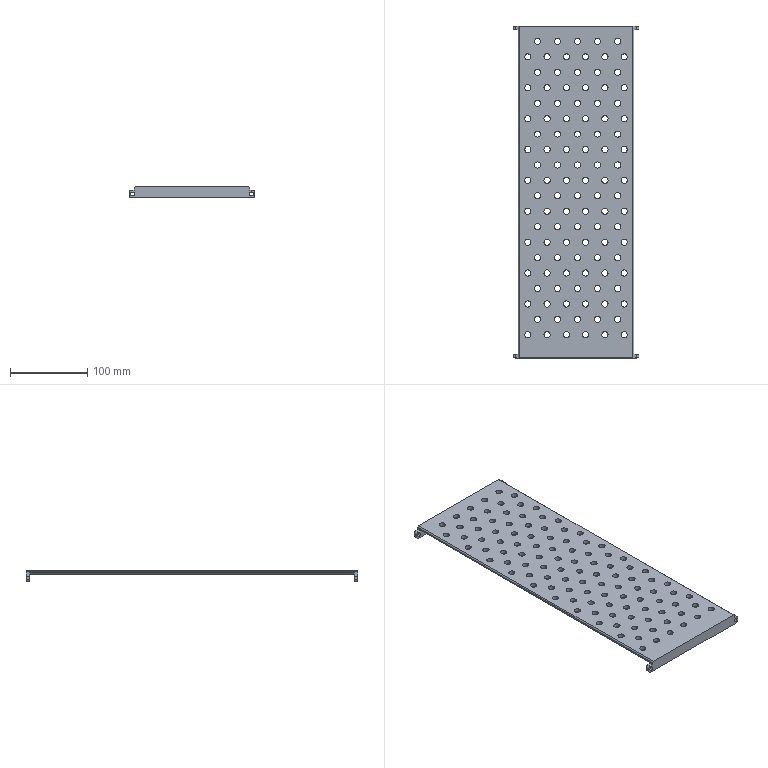Part | SolidWorks | features ICE 4, Chamfer 1, Extrusion 1, Fillet 1, LPattern 1 | 1 solid | 258 faces | box 163 x 430 x 15 mm | volume 308772 mm3 | cylinder 236 | plane 22 | commonest cylinder face diameters 8 x220 5 x8 6 x8